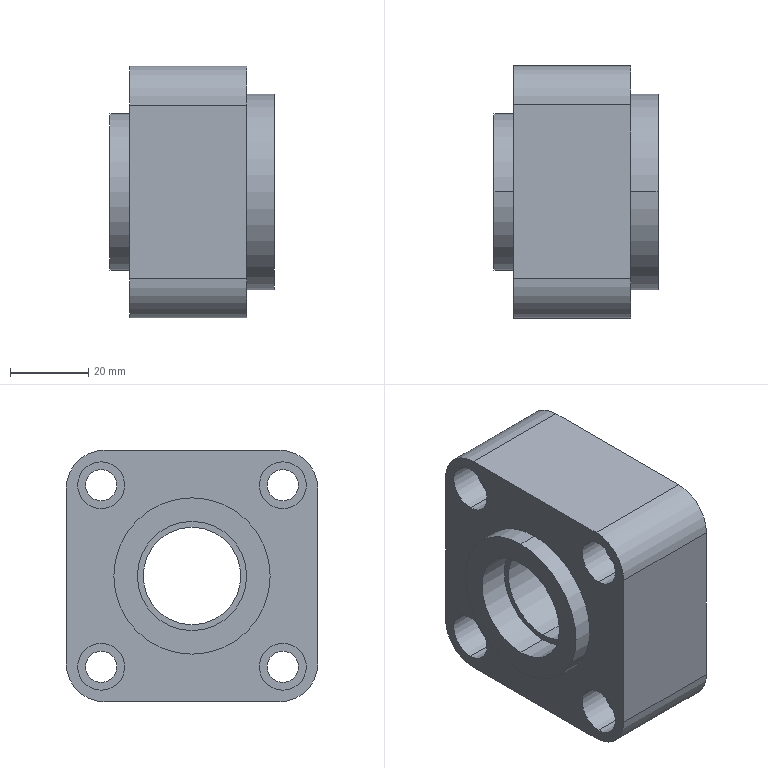Part | STEP file | 1 solid | 44 faces | box 42 x 64.5 x 64.5 mm | volume 111603 mm3 | cylinder 30 | plane 14 | commonest cylinder face diameters 8 x8 12 x8 20 x4 28 x4 25 x2 40 x2
STEP:
#1=CARTESIAN_POINT('',(-20.091,0.,-20.));
#2=VERTEX_POINT('',#1);
#3=CARTESIAN_POINT('',(-20.091,0.,20.));
#4=VERTEX_POINT('',#3);
#5=CARTESIAN_POINT('',(-20.091,0.,0.));
#6=DIRECTION('',(1.,0.,0.));
#7=DIRECTION('',(0.,0.,-1.));
#8=AXIS2_PLACEMENT_3D('',#5,#6,#7);
#9=CIRCLE('',#8,20.);
#10=EDGE_CURVE('',#2,#4,#9,.T.);
#11=ORIENTED_EDGE('',*,*,#10,.T.);
#12=CARTESIAN_POINT('',(-15.091,0.,20.));
#13=VERTEX_POINT('',#12);
#14=CARTESIAN_POINT('',(-20.091,0.,20.));
#15=DIRECTION('',(1.,0.,0.));
#16=VECTOR('',#15,1000.);
#17=LINE('',#14,#16);
#18=EDGE_CURVE('',#4,#13,#17,.T.);
#19=ORIENTED_EDGE('',*,*,#18,.T.);
#20=CARTESIAN_POINT('',(-15.091,0.,-20.));
#21=VERTEX_POINT('',#20);
#22=CARTESIAN_POINT('',(-15.091,0.,0.));
#23=DIRECTION('',(1.,0.,0.));
#24=DIRECTION('',(0.,0.,-1.));
#25=AXIS2_PLACEMENT_3D('',#22,#23,#24);
#26=CIRCLE('',#25,20.);
#27=EDGE_CURVE('',#21,#13,#26,.T.);
#28=ORIENTED_EDGE('',*,*,#27,.F.);
#29=CARTESIAN_POINT('',(-20.091,0.,-20.));
#30=DIRECTION('',(1.,0.,0.));
#31=VECTOR('',#30,1000.);
#32=LINE('',#29,#31);
#33=EDGE_CURVE('',#2,#21,#32,.T.);
#34=ORIENTED_EDGE('',*,*,#33,.F.);
#35=EDGE_LOOP('',(#11,#19,#28,#34));
#36=FACE_OUTER_BOUND('',#35,.T.);
#37=CARTESIAN_POINT('',(-20.091,0.,0.));
#38=DIRECTION('',(1.,0.,0.));
#39=DIRECTION('',(0.,0.,-1.));
#40=AXIS2_PLACEMENT_3D('',#37,#38,#39);
#41=CYLINDRICAL_SURFACE('',#40,20.);
#42=ADVANCED_FACE('',(#36),#41,.T.);
#43=CARTESIAN_POINT('',(-15.091,23.25,29.25));
#44=VERTEX_POINT('',#43);
#45=CARTESIAN_POINT('',(-15.091,23.25,17.25));
#46=VERTEX_POINT('',#45);
#47=CARTESIAN_POINT('',(-15.091,23.25,23.25));
#48=DIRECTION('',(1.,0.,0.));
#49=DIRECTION('',(0.,0.,-1.));
#50=AXIS2_PLACEMENT_3D('',#47,#48,#49);
#51=CIRCLE('',#50,6.);
#52=EDGE_CURVE('',#44,#46,#51,.T.);
#53=ORIENTED_EDGE('',*,*,#52,.F.);
#54=CARTESIAN_POINT('',(-7.091,23.25,29.25));
#55=VERTEX_POINT('',#54);
#56=CARTESIAN_POINT('',(-15.091,23.25,29.25));
#57=DIRECTION('',(1.,0.,0.));
#58=VECTOR('',#57,1000.);
#59=LINE('',#56,#58);
#60=EDGE_CURVE('',#44,#55,#59,.T.);
#61=ORIENTED_EDGE('',*,*,#60,.T.);
#62=CARTESIAN_POINT('',(-7.091,23.25,17.25));
#63=VERTEX_POINT('',#62);
#64=CARTESIAN_POINT('',(-7.091,23.25,23.25));
#65=DIRECTION('',(-1.,0.,0.));
#66=DIRECTION('',(0.,0.,-1.));
#67=AXIS2_PLACEMENT_3D('',#64,#65,#66);
#68=CIRCLE('',#67,6.);
#69=EDGE_CURVE('',#63,#55,#68,.T.);
#70=ORIENTED_EDGE('',*,*,#69,.F.);
#71=CARTESIAN_POINT('',(-15.091,23.25,17.25));
#72=DIRECTION('',(1.,0.,0.));
#73=VECTOR('',#72,1000.);
#74=LINE('',#71,#73);
#75=EDGE_CURVE('',#46,#63,#74,.T.);
#76=ORIENTED_EDGE('',*,*,#75,.F.);
#77=EDGE_LOOP('',(#53,#61,#70,#76));
#78=FACE_OUTER_BOUND('',#77,.T.);
#79=CARTESIAN_POINT('',(-15.091,23.25,23.25));
#80=DIRECTION('',(1.,0.,0.));
#81=DIRECTION('',(0.,0.,-1.));
#82=AXIS2_PLACEMENT_3D('',#79,#80,#81);
#83=CYLINDRICAL_SURFACE('',#82,6.);
#84=ADVANCED_FACE('',(#78),#83,.F.);
#85=CARTESIAN_POINT('',(-15.091,23.25,-17.25));
#86=VERTEX_POINT('',#85);
#87=CARTESIAN_POINT('',(-15.091,23.25,-29.25));
#88=VERTEX_POINT('',#87);
#89=CARTESIAN_POINT('',(-15.091,23.25,-23.25));
#90=DIRECTION('',(1.,0.,0.));
#91=DIRECTION('',(0.,0.,-1.));
#92=AXIS2_PLACEMENT_3D('',#89,#90,#91);
#93=CIRCLE('',#92,6.);
#94=EDGE_CURVE('',#86,#88,#93,.T.);
#95=ORIENTED_EDGE('',*,*,#94,.F.);
#96=CARTESIAN_POINT('',(-7.091,23.25,-17.25));
#97=VERTEX_POINT('',#96);
#98=CARTESIAN_POINT('',(-15.091,23.25,-17.25));
#99=DIRECTION('',(1.,0.,0.));
#100=VECTOR('',#99,1000.);
#101=LINE('',#98,#100);
#102=EDGE_CURVE('',#86,#97,#101,.T.);
#103=ORIENTED_EDGE('',*,*,#102,.T.);
#104=CARTESIAN_POINT('',(-7.091,23.25,-29.25));
#105=VERTEX_POINT('',#104);
#106=CARTESIAN_POINT('',(-7.091,23.25,-23.25));
#107=DIRECTION('',(-1.,0.,0.));
#108=DIRECTION('',(0.,0.,-1.));
#109=AXIS2_PLACEMENT_3D('',#106,#107,#108);
#110=CIRCLE('',#109,6.);
#111=EDGE_CURVE('',#105,#97,#110,.T.);
#112=ORIENTED_EDGE('',*,*,#111,.F.);
#113=CARTESIAN_POINT('',(-15.091,23.25,-29.25));
#114=DIRECTION('',(1.,0.,0.));
#115=VECTOR('',#114,1000.);
#116=LINE('',#113,#115);
#117=EDGE_CURVE('',#88,#105,#116,.T.);
#118=ORIENTED_EDGE('',*,*,#117,.F.);
#119=EDGE_LOOP('',(#95,#103,#112,#118));
#120=FACE_OUTER_BOUND('',#119,.T.);
#121=CARTESIAN_POINT('',(-15.091,23.25,-23.25));
#122=DIRECTION('',(1.,0.,0.));
#123=DIRECTION('',(0.,0.,-1.));
#124=AXIS2_PLACEMENT_3D('',#121,#122,#123);
#125=CYLINDRICAL_SURFACE('',#124,6.);
#126=ADVANCED_FACE('',(#120),#125,.F.);
#127=CARTESIAN_POINT('',(-15.091,-23.25,-17.25));
#128=VERTEX_POINT('',#127);
#129=CARTESIAN_POINT('',(-15.091,-23.25,-29.25));
#130=VERTEX_POINT('',#129);
#131=CARTESIAN_POINT('',(-15.091,-23.25,-23.25));
#132=DIRECTION('',(1.,0.,0.));
#133=DIRECTION('',(0.,0.,-1.));
#134=AXIS2_PLACEMENT_3D('',#131,#132,#133);
#135=CIRCLE('',#134,6.);
#136=EDGE_CURVE('',#128,#130,#135,.T.);
#137=ORIENTED_EDGE('',*,*,#136,.F.);
#138=CARTESIAN_POINT('',(-7.091,-23.25,-17.25));
#139=VERTEX_POINT('',#138);
#140=CARTESIAN_POINT('',(-15.091,-23.25,-17.25));
#141=DIRECTION('',(1.,0.,0.));
#142=VECTOR('',#141,1000.);
#143=LINE('',#140,#142);
#144=EDGE_CURVE('',#128,#139,#143,.T.);
#145=ORIENTED_EDGE('',*,*,#144,.T.);
#146=CARTESIAN_POINT('',(-7.091,-23.25,-29.25));
#147=VERTEX_POINT('',#146);
#148=CARTESIAN_POINT('',(-7.091,-23.25,-23.25));
#149=DIRECTION('',(-1.,0.,0.));
#150=DIRECTION('',(0.,0.,-1.));
#151=AXIS2_PLACEMENT_3D('',#148,#149,#150);
#152=CIRCLE('',#151,6.);
#153=EDGE_CURVE('',#147,#139,#152,.T.);
#154=ORIENTED_EDGE('',*,*,#153,.F.);
#155=CARTESIAN_POINT('',(-15.091,-23.25,-29.25));
#156=DIRECTION('',(1.,0.,0.));
#157=VECTOR('',#156,1000.);
#158=LINE('',#155,#157);
#159=EDGE_CURVE('',#130,#147,#158,.T.);
#160=ORIENTED_EDGE('',*,*,#159,.F.);
#161=EDGE_LOOP('',(#137,#145,#154,#160));
#162=FACE_OUTER_BOUND('',#161,.T.);
#163=CARTESIAN_POINT('',(-15.091,-23.25,-23.25));
#164=DIRECTION('',(1.,0.,0.));
#165=DIRECTION('',(0.,0.,-1.));
#166=AXIS2_PLACEMENT_3D('',#163,#164,#165);
#167=CYLINDRICAL_SURFACE('',#166,6.);
#168=ADVANCED_FACE('',(#162),#167,.F.);
#169=CARTESIAN_POINT('',(-15.091,-23.25,29.25));
#170=VERTEX_POINT('',#169);
#171=CARTESIAN_POINT('',(-15.091,-23.25,17.25));
#172=VERTEX_POINT('',#171);
#173=CARTESIAN_POINT('',(-15.091,-23.25,23.25));
#174=DIRECTION('',(1.,0.,0.));
#175=DIRECTION('',(0.,0.,-1.));
#176=AXIS2_PLACEMENT_3D('',#173,#174,#175);
#177=CIRCLE('',#176,6.);
#178=EDGE_CURVE('',#170,#172,#177,.T.);
#179=ORIENTED_EDGE('',*,*,#178,.F.);
#180=CARTESIAN_POINT('',(-7.091,-23.25,29.25));
#181=VERTEX_POINT('',#180);
#182=CARTESIAN_POINT('',(-15.091,-23.25,29.25));
#183=DIRECTION('',(1.,0.,0.));
#184=VECTOR('',#183,1000.);
#185=LINE('',#182,#184);
#186=EDGE_CURVE('',#170,#181,#185,.T.);
#187=ORIENTED_EDGE('',*,*,#186,.T.);
#188=CARTESIAN_POINT('',(-7.091,-23.25,17.25));
#189=VERTEX_POINT('',#188);
#190=CARTESIAN_POINT('',(-7.091,-23.25,23.25));
#191=DIRECTION('',(-1.,0.,0.));
#192=DIRECTION('',(0.,0.,-1.));
#193=AXIS2_PLACEMENT_3D('',#190,#191,#192);
#194=CIRCLE('',#193,6.);
#195=EDGE_CURVE('',#189,#181,#194,.T.);
#196=ORIENTED_EDGE('',*,*,#195,.F.);
#197=CARTESIAN_POINT('',(-15.091,-23.25,17.25));
#198=DIRECTION('',(1.,0.,0.));
#199=VECTOR('',#198,1000.);
#200=LINE('',#197,#199);
#201=EDGE_CURVE('',#172,#189,#200,.T.);
#202=ORIENTED_EDGE('',*,*,#201,.F.);
#203=EDGE_LOOP('',(#179,#187,#196,#202));
#204=FACE_OUTER_BOUND('',#203,.T.);
#205=CARTESIAN_POINT('',(-15.091,-23.25,23.25));
#206=DIRECTION('',(1.,0.,0.));
#207=DIRECTION('',(0.,0.,-1.));
#208=AXIS2_PLACEMENT_3D('',#205,#206,#207);
#209=CYLINDRICAL_SURFACE('',#208,6.);
#210=ADVANCED_FACE('',(#204),#209,.F.);
#211=CARTESIAN_POINT('',(14.909,0.,25.));
#212=VERTEX_POINT('',#211);
#213=CARTESIAN_POINT('',(14.909,0.,-25.));
#214=VERTEX_POINT('',#213);
#215=CARTESIAN_POINT('',(14.909,0.,0.));
#216=DIRECTION('',(-1.,0.,0.));
#217=DIRECTION('',(0.,0.,-1.));
#218=AXIS2_PLACEMENT_3D('',#215,#216,#217);
#219=CIRCLE('',#218,25.);
#220=EDGE_CURVE('',#212,#214,#219,.T.);
#221=ORIENTED_EDGE('',*,*,#220,.F.);
#222=CARTESIAN_POINT('',(21.909,0.,25.));
#223=VERTEX_POINT('',#222);
#224=CARTESIAN_POINT('',(14.909,0.,25.));
#225=DIRECTION('',(1.,0.,0.));
#226=VECTOR('',#225,1000.);
#227=LINE('',#224,#226);
#228=EDGE_CURVE('',#212,#223,#227,.T.);
#229=ORIENTED_EDGE('',*,*,#228,.T.);
#230=CARTESIAN_POINT('',(21.909,0.,-25.));
#231=VERTEX_POINT('',#230);
#232=CARTESIAN_POINT('',(21.909,0.,0.));
#233=DIRECTION('',(-1.,0.,0.));
#234=DIRECTION('',(0.,0.,-1.));
#235=AXIS2_PLACEMENT_3D('',#232,#233,#234);
#236=CIRCLE('',#235,25.);
#237=EDGE_CURVE('',#223,#231,#236,.T.);
#238=ORIENTED_EDGE('',*,*,#237,.T.);
#239=CARTESIAN_POINT('',(14.909,0.,-25.));
#240=DIRECTION('',(1.,0.,0.));
#241=VECTOR('',#240,1000.);
#242=LINE('',#239,#241);
#243=EDGE_CURVE('',#214,#231,#242,.T.);
#244=ORIENTED_EDGE('',*,*,#243,.F.);
#245=EDGE_LOOP('',(#221,#229,#238,#244));
#246=FACE_OUTER_BOUND('',#245,.T.);
#247=CARTESIAN_POINT('',(14.909,0.,0.));
#248=DIRECTION('',(1.,0.,0.));
#249=DIRECTION('',(0.,0.,-1.));
#250=AXIS2_PLACEMENT_3D('',#247,#248,#249);
#251=CYLINDRICAL_SURFACE('',#250,25.);
#252=ADVANCED_FACE('',(#246),#251,.T.);
#253=CARTESIAN_POINT('',(-7.091,23.25,19.25));
#254=VERTEX_POINT('',#253);
#255=CARTESIAN_POINT('',(-7.091,23.25,27.25));
#256=VERTEX_POINT('',#255);
#257=CARTESIAN_POINT('',(-7.091,23.25,23.25));
#258=DIRECTION('',(-1.,0.,0.));
#259=DIRECTION('',(0.,0.,-1.));
#260=AXIS2_PLACEMENT_3D('',#257,#258,#259);
#261=CIRCLE('',#260,4.);
#262=EDGE_CURVE('',#254,#256,#261,.T.);
#263=ORIENTED_EDGE('',*,*,#262,.T.);
#264=CARTESIAN_POINT('',(14.909,23.25,27.25));
#265=VERTEX_POINT('',#264);
#266=CARTESIAN_POINT('',(-7.091,23.25,27.25));
#267=DIRECTION('',(1.,0.,0.));
#268=VECTOR('',#267,1000.);
#269=LINE('',#266,#268);
#270=EDGE_CURVE('',#256,#265,#269,.T.);
#271=ORIENTED_EDGE('',*,*,#270,.T.);
#272=CARTESIAN_POINT('',(14.909,23.25,19.25));
#273=VERTEX_POINT('',#272);
#274=CARTESIAN_POINT('',(14.909,23.25,23.25));
#275=DIRECTION('',(-1.,0.,0.));
#276=DIRECTION('',(0.,0.,-1.));
#277=AXIS2_PLACEMENT_3D('',#274,#275,#276);
#278=CIRCLE('',#277,4.);
#279=EDGE_CURVE('',#273,#265,#278,.T.);
#280=ORIENTED_EDGE('',*,*,#279,.F.);
#281=CARTESIAN_POINT('',(-7.091,23.25,19.25));
#282=DIRECTION('',(1.,0.,0.));
#283=VECTOR('',#282,1000.);
#284=LINE('',#281,#283);
#285=EDGE_CURVE('',#254,#273,#284,.T.);
#286=ORIENTED_EDGE('',*,*,#285,.F.);
#287=EDGE_LOOP('',(#263,#271,#280,#286));
#288=FACE_OUTER_BOUND('',#287,.T.);
#289=CARTESIAN_POINT('',(-7.091,23.25,23.25));
#290=DIRECTION('',(1.,0.,0.));
#291=DIRECTION('',(0.,0.,-1.));
#292=AXIS2_PLACEMENT_3D('',#289,#290,#291);
#293=CYLINDRICAL_SURFACE('',#292,4.);
#294=ADVANCED_FACE('',(#288),#293,.F.);
#295=CARTESIAN_POINT('',(-7.091,23.25,-27.25));
#296=VERTEX_POINT('',#295);
#297=CARTESIAN_POINT('',(-7.091,23.25,-19.25));
#298=VERTEX_POINT('',#297);
#299=CARTESIAN_POINT('',(-7.091,23.25,-23.25));
#300=DIRECTION('',(-1.,0.,0.));
#301=DIRECTION('',(0.,0.,-1.));
#302=AXIS2_PLACEMENT_3D('',#299,#300,#301);
#303=CIRCLE('',#302,4.);
#304=EDGE_CURVE('',#296,#298,#303,.T.);
#305=ORIENTED_EDGE('',*,*,#304,.T.);
#306=CARTESIAN_POINT('',(14.909,23.25,-19.25));
#307=VERTEX_POINT('',#306);
#308=CARTESIAN_POINT('',(-7.091,23.25,-19.25));
#309=DIRECTION('',(1.,0.,0.));
#310=VECTOR('',#309,1000.);
#311=LINE('',#308,#310);
#312=EDGE_CURVE('',#298,#307,#311,.T.);
#313=ORIENTED_EDGE('',*,*,#312,.T.);
#314=CARTESIAN_POINT('',(14.909,23.25,-27.25));
#315=VERTEX_POINT('',#314);
#316=CARTESIAN_POINT('',(14.909,23.25,-23.25));
#317=DIRECTION('',(-1.,0.,0.));
#318=DIRECTION('',(0.,0.,-1.));
#319=AXIS2_PLACEMENT_3D('',#316,#317,#318);
#320=CIRCLE('',#319,4.);
#321=EDGE_CURVE('',#315,#307,#320,.T.);
#322=ORIENTED_EDGE('',*,*,#321,.F.);
#323=CARTESIAN_POINT('',(-7.091,23.25,-27.25));
#324=DIRECTION('',(1.,0.,0.));
#325=VECTOR('',#324,1000.);
#326=LINE('',#323,#325);
#327=EDGE_CURVE('',#296,#315,#326,.T.);
#328=ORIENTED_EDGE('',*,*,#327,.F.);
#329=EDGE_LOOP('',(#305,#313,#322,#328));
#330=FACE_OUTER_BOUND('',#329,.T.);
#331=CARTESIAN_POINT('',(-7.091,23.25,-23.25));
#332=DIRECTION('',(1.,0.,0.));
#333=DIRECTION('',(0.,0.,-1.));
#334=AXIS2_PLACEMENT_3D('',#331,#332,#333);
#335=CYLINDRICAL_SURFACE('',#334,4.);
#336=ADVANCED_FACE('',(#330),#335,.F.);
#337=CARTESIAN_POINT('',(-7.091,-23.25,-27.25));
#338=VERTEX_POINT('',#337);
#339=CARTESIAN_POINT('',(-7.091,-23.25,-19.25));
#340=VERTEX_POINT('',#339);
#341=CARTESIAN_POINT('',(-7.091,-23.25,-23.25));
#342=DIRECTION('',(-1.,0.,0.));
#343=DIRECTION('',(0.,0.,-1.));
#344=AXIS2_PLACEMENT_3D('',#341,#342,#343);
#345=CIRCLE('',#344,4.);
#346=EDGE_CURVE('',#338,#340,#345,.T.);
#347=ORIENTED_EDGE('',*,*,#346,.T.);
#348=CARTESIAN_POINT('',(14.909,-23.25,-19.25));
#349=VERTEX_POINT('',#348);
#350=CARTESIAN_POINT('',(-7.091,-23.25,-19.25));
#351=DIRECTION('',(1.,0.,0.));
#352=VECTOR('',#351,1000.);
#353=LINE('',#350,#352);
#354=EDGE_CURVE('',#340,#349,#353,.T.);
#355=ORIENTED_EDGE('',*,*,#354,.T.);
#356=CARTESIAN_POINT('',(14.909,-23.25,-27.25));
#357=VERTEX_POINT('',#356);
#358=CARTESIAN_POINT('',(14.909,-23.25,-23.25));
#359=DIRECTION('',(-1.,0.,0.));
#360=DIRECTION('',(0.,0.,-1.));
#361=AXIS2_PLACEMENT_3D('',#358,#359,#360);
#362=CIRCLE('',#361,4.);
#363=EDGE_CURVE('',#357,#349,#362,.T.);
#364=ORIENTED_EDGE('',*,*,#363,.F.);
#365=CARTESIAN_POINT('',(-7.091,-23.25,-27.25));
#366=DIRECTION('',(1.,0.,0.));
#367=VECTOR('',#366,1000.);
#368=LINE('',#365,#367);
#369=EDGE_CURVE('',#338,#357,#368,.T.);
#370=ORIENTED_EDGE('',*,*,#369,.F.);
#371=EDGE_LOOP('',(#347,#355,#364,#370));
#372=FACE_OUTER_BOUND('',#371,.T.);
#373=CARTESIAN_POINT('',(-7.091,-23.25,-23.25));
#374=DIRECTION('',(1.,0.,0.));
#375=DIRECTION('',(0.,0.,-1.));
#376=AXIS2_PLACEMENT_3D('',#373,#374,#375);
#377=CYLINDRICAL_SURFACE('',#376,4.);
#378=ADVANCED_FACE('',(#372),#377,.F.);
#379=CARTESIAN_POINT('',(-7.091,-23.25,19.25));
#380=VERTEX_POINT('',#379);
#381=CARTESIAN_POINT('',(-7.091,-23.25,27.25));
#382=VERTEX_POINT('',#381);
#383=CARTESIAN_POINT('',(-7.091,-23.25,23.25));
#384=DIRECTION('',(-1.,0.,0.));
#385=DIRECTION('',(0.,0.,-1.));
#386=AXIS2_PLACEMENT_3D('',#383,#384,#385);
#387=CIRCLE('',#386,4.);
#388=EDGE_CURVE('',#380,#382,#387,.T.);
#389=ORIENTED_EDGE('',*,*,#388,.T.);
#390=CARTESIAN_POINT('',(14.909,-23.25,27.25));
#391=VERTEX_POINT('',#390);
#392=CARTESIAN_POINT('',(-7.091,-23.25,27.25));
#393=DIRECTION('',(1.,0.,0.));
#394=VECTOR('',#393,1000.);
#395=LINE('',#392,#394);
#396=EDGE_CURVE('',#382,#391,#395,.T.);
#397=ORIENTED_EDGE('',*,*,#396,.T.);
#398=CARTESIAN_POINT('',(14.909,-23.25,19.25));
#399=VERTEX_POINT('',#398);
#400=CARTESIAN_POINT('',(14.909,-23.25,23.25));
#401=DIRECTION('',(-1.,0.,0.));
#402=DIRECTION('',(0.,0.,-1.));
#403=AXIS2_PLACEMENT_3D('',#400,#401,#402);
#404=CIRCLE('',#403,4.);
#405=EDGE_CURVE('',#399,#391,#404,.T.);
#406=ORIENTED_EDGE('',*,*,#405,.F.);
#407=CARTESIAN_POINT('',(-7.091,-23.25,19.25));
#408=DIRECTION('',(1.,0.,0.));
#409=VECTOR('',#408,1000.);
#410=LINE('',#407,#409);
#411=EDGE_CURVE('',#380,#399,#410,.T.);
#412=ORIENTED_EDGE('',*,*,#411,.F.);
#413=EDGE_LOOP('',(#389,#397,#406,#412));
#414=FACE_OUTER_BOUND('',#413,.T.);
#415=CARTESIAN_POINT('',(-7.091,-23.25,23.25));
#416=DIRECTION('',(1.,0.,0.));
#417=DIRECTION('',(0.,0.,-1.));
#418=AXIS2_PLACEMENT_3D('',#415,#416,#417);
#419=CYLINDRICAL_SURFACE('',#418,4.);
#420=ADVANCED_FACE('',(#414),#419,.F.);
#421=CARTESIAN_POINT('',(-20.091,0.,14.));
#422=VERTEX_POINT('',#421);
#423=CARTESIAN_POINT('',(-20.091,0.,-14.));
#424=VERTEX_POINT('',#423);
#425=CARTESIAN_POINT('',(-20.091,0.,0.));
#426=DIRECTION('',(1.,0.,0.));
#427=DIRECTION('',(0.,0.,-1.));
#428=AXIS2_PLACEMENT_3D('',#425,#426,#427);
#429=CIRCLE('',#428,14.);
#430=EDGE_CURVE('',#422,#424,#429,.T.);
#431=ORIENTED_EDGE('',*,*,#430,.F.);
#432=CARTESIAN_POINT('',(-12.091,0.,14.));
#433=VERTEX_POINT('',#432);
#434=CARTESIAN_POINT('',(-20.091,0.,14.));
#435=DIRECTION('',(1.,0.,0.));
#436=VECTOR('',#435,1000.);
#437=LINE('',#434,#436);
#438=EDGE_CURVE('',#422,#433,#437,.T.);
#439=ORIENTED_EDGE('',*,*,#438,.T.);
#440=CARTESIAN_POINT('',(-12.091,0.,-14.));
#441=VERTEX_POINT('',#440);
#442=CARTESIAN_POINT('',(-12.091,0.,0.));
#443=DIRECTION('',(-1.,0.,0.));
#444=DIRECTION('',(0.,0.,-1.));
#445=AXIS2_PLACEMENT_3D('',#442,#443,#444);
#446=CIRCLE('',#445,14.);
#447=EDGE_CURVE('',#441,#433,#446,.T.);
#448=ORIENTED_EDGE('',*,*,#447,.F.);
#449=CARTESIAN_POINT('',(-20.091,0.,-14.));
#450=DIRECTION('',(1.,0.,0.));
#451=VECTOR('',#450,1000.);
#452=LINE('',#449,#451);
#453=EDGE_CURVE('',#424,#441,#452,.T.);
#454=ORIENTED_EDGE('',*,*,#453,.F.);
#455=EDGE_LOOP('',(#431,#439,#448,#454));
#456=FACE_OUTER_BOUND('',#455,.T.);
#457=CARTESIAN_POINT('',(-20.091,0.,0.));
#458=DIRECTION('',(1.,0.,0.));
#459=DIRECTION('',(0.,0.,-1.));
#460=AXIS2_PLACEMENT_3D('',#457,#458,#459);
#461=CYLINDRICAL_SURFACE('',#460,14.);
#462=ADVANCED_FACE('',(#456),#461,.F.);
#463=CARTESIAN_POINT('',(13.909,0.,14.));
#464=VERTEX_POINT('',#463);
#465=CARTESIAN_POINT('',(13.909,0.,-14.));
#466=VERTEX_POINT('',#465);
#467=CARTESIAN_POINT('',(13.909,0.,0.));
#468=DIRECTION('',(1.,0.,0.));
#469=DIRECTION('',(0.,0.,-1.));
#470=AXIS2_PLACEMENT_3D('',#467,#468,#469);
#471=CIRCLE('',#470,14.);
#472=EDGE_CURVE('',#464,#466,#471,.T.);
#473=ORIENTED_EDGE('',*,*,#472,.F.);
#474=CARTESIAN_POINT('',(21.909,0.,14.));
#475=VERTEX_POINT('',#474);
#476=CARTESIAN_POINT('',(13.909,0.,14.));
#477=DIRECTION('',(1.,0.,0.));
#478=VECTOR('',#477,1000.);
#479=LINE('',#476,#478);
#480=EDGE_CURVE('',#464,#475,#479,.T.);
#481=ORIENTED_EDGE('',*,*,#480,.T.);
#482=CARTESIAN_POINT('',(21.909,0.,-14.));
#483=VERTEX_POINT('',#482);
#484=CARTESIAN_POINT('',(21.909,0.,0.));
#485=DIRECTION('',(-1.,0.,0.));
#486=DIRECTION('',(0.,0.,-1.));
#487=AXIS2_PLACEMENT_3D('',#484,#485,#486);
#488=CIRCLE('',#487,14.);
#489=EDGE_CURVE('',#483,#475,#488,.T.);
#490=ORIENTED_EDGE('',*,*,#489,.F.);
#491=CARTESIAN_POINT('',(13.909,0.,-14.));
#492=DIRECTION('',(1.,0.,0.));
#493=VECTOR('',#492,1000.);
#494=LINE('',#491,#493);
#495=EDGE_CURVE('',#466,#483,#494,.T.);
#496=ORIENTED_EDGE('',*,*,#495,.F.);
#497=EDGE_LOOP('',(#473,#481,#490,#496));
#498=FACE_OUTER_BOUND('',#497,.T.);
#499=CARTESIAN_POINT('',(13.909,0.,0.));
#500=DIRECTION('',(1.,0.,0.));
#501=DIRECTION('',(0.,0.,-1.));
#502=AXIS2_PLACEMENT_3D('',#499,#500,#501);
#503=CYLINDRICAL_SURFACE('',#502,14.);
#504=ADVANCED_FACE('',(#498),#503,.F.);
#505=CARTESIAN_POINT('',(-12.091,0.,-12.5));
#506=VERTEX_POINT('',#505);
#507=CARTESIAN_POINT('',(-12.091,0.,12.5));
#508=VERTEX_POINT('',#507);
#509=CARTESIAN_POINT('',(-12.091,0.,0.));
#510=DIRECTION('',(-1.,0.,0.));
#511=DIRECTION('',(0.,0.,-1.));
#512=AXIS2_PLACEMENT_3D('',#509,#510,#511);
#513=CIRCLE('',#512,12.5);
#514=EDGE_CURVE('',#506,#508,#513,.T.);
#515=ORIENTED_EDGE('',*,*,#514,.T.);
#516=CARTESIAN_POINT('',(13.909,0.,12.5));
#517=VERTEX_POINT('',#516);
#518=CARTESIAN_POINT('',(-12.091,0.,12.5));
#519=DIRECTION('',(1.,0.,0.));
#520=VECTOR('',#519,1000.);
#521=LINE('',#518,#520);
#522=EDGE_CURVE('',#508,#517,#521,.T.);
#523=ORIENTED_EDGE('',*,*,#522,.T.);
#524=CARTESIAN_POINT('',(13.909,0.,-12.5));
#525=VERTEX_POINT('',#524);
#526=CARTESIAN_POINT('',(13.909,0.,0.));
#527=DIRECTION('',(-1.,0.,0.));
#528=DIRECTION('',(0.,0.,-1.));
#529=AXIS2_PLACEMENT_3D('',#526,#527,#528);
#530=CIRCLE('',#529,12.5);
#531=EDGE_CURVE('',#525,#517,#530,.T.);
#532=ORIENTED_EDGE('',*,*,#531,.F.);
#533=CARTESIAN_POINT('',(-12.091,0.,-12.5));
#534=DIRECTION('',(1.,0.,0.));
#535=VECTOR('',#534,1000.);
#536=LINE('',#533,#535);
#537=EDGE_CURVE('',#506,#525,#536,.T.);
#538=ORIENTED_EDGE('',*,*,#537,.F.);
#539=EDGE_LOOP('',(#515,#523,#532,#538));
#540=FACE_OUTER_BOUND('',#539,.T.);
#541=CARTESIAN_POINT('',(-12.091,0.,0.));
#542=DIRECTION('',(1.,0.,0.));
#543=DIRECTION('',(0.,0.,-1.));
#544=AXIS2_PLACEMENT_3D('',#541,#542,#543);
#545=CYLINDRICAL_SURFACE('',#544,12.5);
#546=ADVANCED_FACE('',(#540),#545,.F.);
#547=CARTESIAN_POINT('',(-15.091,-22.25,-32.25));
#548=VERTEX_POINT('',#547);
#549=CARTESIAN_POINT('',(-15.091,-32.25,-22.25));
#550=VERTEX_POINT('',#549);
#551=CARTESIAN_POINT('',(-15.091,-22.25,-22.25));
#552=DIRECTION('',(-1.,0.,0.));
#553=DIRECTION('',(0.,0.,-1.));
#554=AXIS2_PLACEMENT_3D('',#551,#552,#553);
#555=CIRCLE('',#554,10.);
#556=EDGE_CURVE('',#548,#550,#555,.T.);
#557=ORIENTED_EDGE('',*,*,#556,.T.);
#558=CARTESIAN_POINT('',(-15.091,-32.25,22.25));
#559=VERTEX_POINT('',#558);
#560=CARTESIAN_POINT('',(-15.091,-32.25,-32.25));
#561=DIRECTION('',(0.,0.,1.));
#562=VECTOR('',#561,1000.);
#563=LINE('',#560,#562);
#564=EDGE_CURVE('',#550,#559,#563,.T.);
#565=ORIENTED_EDGE('',*,*,#564,.T.);
#566=CARTESIAN_POINT('',(-15.091,-22.25,32.25));
#567=VERTEX_POINT('',#566);
#568=CARTESIAN_POINT('',(-15.091,-22.25,22.25));
#569=DIRECTION('',(-1.,0.,0.));
#570=DIRECTION('',(0.,0.,-1.));
#571=AXIS2_PLACEMENT_3D('',#568,#569,#570);
#572=CIRCLE('',#571,10.);
#573=EDGE_CURVE('',#559,#567,#572,.T.);
#574=ORIENTED_EDGE('',*,*,#573,.T.);
#575=CARTESIAN_POINT('',(-15.091,22.25,32.25));
#576=VERTEX_POINT('',#575);
#577=CARTESIAN_POINT('',(-15.091,-32.25,32.25));
#578=DIRECTION('',(0.,1.,0.));
#579=VECTOR('',#578,1000.);
#580=LINE('',#577,#579);
#581=EDGE_CURVE('',#567,#576,#580,.T.);
#582=ORIENTED_EDGE('',*,*,#581,.T.);
#583=CARTESIAN_POINT('',(-15.091,32.25,22.25));
#584=VERTEX_POINT('',#583);
#585=CARTESIAN_POINT('',(-15.091,22.25,22.25));
#586=DIRECTION('',(-1.,0.,0.));
#587=DIRECTION('',(0.,0.,-1.));
#588=AXIS2_PLACEMENT_3D('',#585,#586,#587);
#589=CIRCLE('',#588,10.);
#590=EDGE_CURVE('',#576,#584,#589,.T.);
#591=ORIENTED_EDGE('',*,*,#590,.T.);
#592=CARTESIAN_POINT('',(-15.091,32.25,-22.25));
#593=VERTEX_POINT('',#592);
#594=CARTESIAN_POINT('',(-15.091,32.25,-32.25));
#595=DIRECTION('',(0.,0.,-1.));
#596=VECTOR('',#595,1000.);
#597=LINE('',#594,#596);
#598=EDGE_CURVE('',#584,#593,#597,.T.);
#599=ORIENTED_EDGE('',*,*,#598,.T.);
#600=CARTESIAN_POINT('',(-15.091,22.25,-32.25));
#601=VERTEX_POINT('',#600);
#602=CARTESIAN_POINT('',(-15.091,22.25,-22.25));
#603=DIRECTION('',(-1.,0.,0.));
#604=DIRECTION('',(0.,0.,-1.));
#605=AXIS2_PLACEMENT_3D('',#602,#603,#604);
#606=CIRCLE('',#605,10.);
#607=EDGE_CURVE('',#593,#601,#606,.T.);
#608=ORIENTED_EDGE('',*,*,#607,.T.);
#609=CARTESIAN_POINT('',(-15.091,-32.25,-32.25));
#610=DIRECTION('',(0.,-1.,0.));
#611=VECTOR('',#610,1000.);
#612=LINE('',#609,#611);
#613=EDGE_CURVE('',#601,#548,#612,.T.);
#614=ORIENTED_EDGE('',*,*,#613,.T.);
#615=EDGE_LOOP('',(#557,#565,#574,#582,#591,#599,#608,#614));
#616=FACE_OUTER_BOUND('',#615,.T.);
#617=ORIENTED_EDGE('',*,*,#27,.T.);
#618=CARTESIAN_POINT('',(-15.091,0.,0.));
#619=DIRECTION('',(1.,0.,0.));
#620=DIRECTION('',(0.,0.,-1.));
#621=AXIS2_PLACEMENT_3D('',#618,#619,#620);
#622=CIRCLE('',#621,20.);
#623=EDGE_CURVE('',#13,#21,#622,.T.);
#624=ORIENTED_EDGE('',*,*,#623,.T.);
#625=EDGE_LOOP('',(#617,#624));
#626=FACE_BOUND('',#625,.T.);
#627=CARTESIAN_POINT('',(-15.091,23.25,23.25));
#628=DIRECTION('',(1.,0.,0.));
#629=DIRECTION('',(0.,0.,-1.));
#630=AXIS2_PLACEMENT_3D('',#627,#628,#629);
#631=CIRCLE('',#630,6.);
#632=EDGE_CURVE('',#46,#44,#631,.T.);
#633=ORIENTED_EDGE('',*,*,#632,.T.);
#634=ORIENTED_EDGE('',*,*,#52,.T.);
#635=EDGE_LOOP('',(#633,#634));
#636=FACE_BOUND('',#635,.T.);
#637=CARTESIAN_POINT('',(-15.091,23.25,-23.25));
#638=DIRECTION('',(1.,0.,0.));
#639=DIRECTION('',(0.,0.,-1.));
#640=AXIS2_PLACEMENT_3D('',#637,#638,#639);
#641=CIRCLE('',#640,6.);
#642=EDGE_CURVE('',#88,#86,#641,.T.);
#643=ORIENTED_EDGE('',*,*,#642,.T.);
#644=ORIENTED_EDGE('',*,*,#94,.T.);
#645=EDGE_LOOP('',(#643,#644));
#646=FACE_BOUND('',#645,.T.);
#647=CARTESIAN_POINT('',(-15.091,-23.25,-23.25));
#648=DIRECTION('',(1.,0.,0.));
#649=DIRECTION('',(0.,0.,-1.));
#650=AXIS2_PLACEMENT_3D('',#647,#648,#649);
#651=CIRCLE('',#650,6.);
#652=EDGE_CURVE('',#130,#128,#651,.T.);
#653=ORIENTED_EDGE('',*,*,#652,.T.);
#654=ORIENTED_EDGE('',*,*,#136,.T.);
#655=EDGE_LOOP('',(#653,#654));
#656=FACE_BOUND('',#655,.T.);
#657=CARTESIAN_POINT('',(-15.091,-23.25,23.25));
#658=DIRECTION('',(1.,0.,0.));
#659=DIRECTION('',(0.,0.,-1.));
#660=AXIS2_PLACEMENT_3D('',#657,#658,#659);
#661=CIRCLE('',#660,6.);
#662=EDGE_CURVE('',#172,#170,#661,.T.);
#663=ORIENTED_EDGE('',*,*,#662,.T.);
#664=ORIENTED_EDGE('',*,*,#178,.T.);
#665=EDGE_LOOP('',(#663,#664));
#666=FACE_BOUND('',#665,.T.);
#667=CARTESIAN_POINT('',(-15.091,-32.25,-32.25));
#668=DIRECTION('',(-1.,0.,0.));
#669=DIRECTION('',(0.,0.,1.));
#670=AXIS2_PLACEMENT_3D('',#667,#668,#669);
#671=PLANE('',#670);
#672=ADVANCED_FACE('',(#616,#626,#636,#646,#656,#666),#671,.T.);
#673=ORIENTED_EDGE('',*,*,#564,.F.);
#674=CARTESIAN_POINT('',(14.909,-32.25,-22.25));
#675=VERTEX_POINT('',#674);
#676=CARTESIAN_POINT('',(-15.091,-32.25,-22.25));
#677=DIRECTION('',(-1.,0.,0.));
#678=VECTOR('',#677,1000.);
#679=LINE('',#676,#678);
#680=EDGE_CURVE('',#675,#550,#679,.T.);
#681=ORIENTED_EDGE('',*,*,#680,.F.);
#682=CARTESIAN_POINT('',(14.909,-32.25,22.25));
#683=VERTEX_POINT('',#682);
#684=CARTESIAN_POINT('',(14.909,-32.25,-22.25));
#685=DIRECTION('',(0.,0.,-1.));
#686=VECTOR('',#685,1000.);
#687=LINE('',#684,#686);
#688=EDGE_CURVE('',#683,#675,#687,.T.);
#689=ORIENTED_EDGE('',*,*,#688,.F.);
#690=CARTESIAN_POINT('',(-15.091,-32.25,22.25));
#691=DIRECTION('',(1.,0.,0.));
#692=VECTOR('',#691,1000.);
#693=LINE('',#690,#692);
#694=EDGE_CURVE('',#559,#683,#693,.T.);
#695=ORIENTED_EDGE('',*,*,#694,.F.);
#696=EDGE_LOOP('',(#673,#681,#689,#695));
#697=FACE_OUTER_BOUND('',#696,.T.);
#698=CARTESIAN_POINT('',(-15.091,-32.25,-22.25));
#699=DIRECTION('',(0.,1.,0.));
#700=DIRECTION('',(1.,0.,0.));
#701=AXIS2_PLACEMENT_3D('',#698,#699,#700);
#702=PLANE('',#701);
#703=ADVANCED_FACE('',(#697),#702,.F.);
#704=ORIENTED_EDGE('',*,*,#556,.F.);
#705=CARTESIAN_POINT('',(14.909,-22.25,-32.25));
#706=VERTEX_POINT('',#705);
#707=CARTESIAN_POINT('',(-15.091,-22.25,-32.25));
#708=DIRECTION('',(1.,0.,0.));
#709=VECTOR('',#708,1000.);
#710=LINE('',#707,#709);
#711=EDGE_CURVE('',#548,#706,#710,.T.);
#712=ORIENTED_EDGE('',*,*,#711,.T.);
#713=CARTESIAN_POINT('',(14.909,-22.25,-22.25));
#714=DIRECTION('',(-1.,0.,0.));
#715=DIRECTION('',(0.,0.,-1.));
#716=AXIS2_PLACEMENT_3D('',#713,#714,#715);
#717=CIRCLE('',#716,10.);
#718=EDGE_CURVE('',#706,#675,#717,.T.);
#719=ORIENTED_EDGE('',*,*,#718,.T.);
#720=ORIENTED_EDGE('',*,*,#680,.T.);
#721=EDGE_LOOP('',(#704,#712,#719,#720));
#722=FACE_OUTER_BOUND('',#721,.T.);
#723=CARTESIAN_POINT('',(-15.091,-22.25,-22.25));
#724=DIRECTION('',(1.,0.,0.));
#725=DIRECTION('',(0.,0.,-1.));
#726=AXIS2_PLACEMENT_3D('',#723,#724,#725);
#727=CYLINDRICAL_SURFACE('',#726,10.);
#728=ADVANCED_FACE('',(#722),#727,.T.);
#729=ORIENTED_EDGE('',*,*,#613,.F.);
#730=CARTESIAN_POINT('',(14.909,22.25,-32.25));
#731=VERTEX_POINT('',#730);
#732=CARTESIAN_POINT('',(-15.091,22.25,-32.25));
#733=DIRECTION('',(-1.,0.,0.));
#734=VECTOR('',#733,1000.);
#735=LINE('',#732,#734);
#736=EDGE_CURVE('',#731,#601,#735,.T.);
#737=ORIENTED_EDGE('',*,*,#736,.F.);
#738=CARTESIAN_POINT('',(14.909,-22.25,-32.25));
#739=DIRECTION('',(0.,1.,0.));
#740=VECTOR('',#739,1000.);
#741=LINE('',#738,#740);
#742=EDGE_CURVE('',#706,#731,#741,.T.);
#743=ORIENTED_EDGE('',*,*,#742,.F.);
#744=ORIENTED_EDGE('',*,*,#711,.F.);
#745=EDGE_LOOP('',(#729,#737,#743,#744));
#746=FACE_OUTER_BOUND('',#745,.T.);
#747=CARTESIAN_POINT('',(-15.091,-22.25,-32.25));
#748=DIRECTION('',(0.,0.,1.));
#749=DIRECTION('',(1.,0.,0.));
#750=AXIS2_PLACEMENT_3D('',#747,#748,#749);
#751=PLANE('',#750);
#752=ADVANCED_FACE('',(#746),#751,.F.);
#753=ORIENTED_EDGE('',*,*,#607,.F.);
#754=CARTESIAN_POINT('',(14.909,32.25,-22.25));
#755=VERTEX_POINT('',#754);
#756=CARTESIAN_POINT('',(-15.091,32.25,-22.25));
#757=DIRECTION('',(1.,0.,0.));
#758=VECTOR('',#757,1000.);
#759=LINE('',#756,#758);
#760=EDGE_CURVE('',#593,#755,#759,.T.);
#761=ORIENTED_EDGE('',*,*,#760,.T.);
#762=CARTESIAN_POINT('',(14.909,22.25,-22.25));
#763=DIRECTION('',(-1.,0.,0.));
#764=DIRECTION('',(0.,0.,-1.));
#765=AXIS2_PLACEMENT_3D('',#762,#763,#764);
#766=CIRCLE('',#765,10.);
#767=EDGE_CURVE('',#755,#731,#766,.T.);
#768=ORIENTED_EDGE('',*,*,#767,.T.);
#769=ORIENTED_EDGE('',*,*,#736,.T.);
#770=EDGE_LOOP('',(#753,#761,#768,#769));
#771=FACE_OUTER_BOUND('',#770,.T.);
#772=CARTESIAN_POINT('',(-15.091,22.25,-22.25));
#773=DIRECTION('',(1.,0.,0.));
#774=DIRECTION('',(0.,0.,-1.));
#775=AXIS2_PLACEMENT_3D('',#772,#773,#774);
#776=CYLINDRICAL_SURFACE('',#775,10.);
#777=ADVANCED_FACE('',(#771),#776,.T.);
#778=CARTESIAN_POINT('',(14.909,32.25,22.25));
#779=VERTEX_POINT('',#778);
#780=CARTESIAN_POINT('',(14.909,32.25,22.25));
#781=DIRECTION('',(0.,0.,1.));
#782=VECTOR('',#781,1000.);
#783=LINE('',#780,#782);
#784=EDGE_CURVE('',#755,#779,#783,.T.);
#785=ORIENTED_EDGE('',*,*,#784,.F.);
#786=ORIENTED_EDGE('',*,*,#760,.F.);
#787=ORIENTED_EDGE('',*,*,#598,.F.);
#788=CARTESIAN_POINT('',(-15.091,32.25,22.25));
#789=DIRECTION('',(-1.,0.,0.));
#790=VECTOR('',#789,1000.);
#791=LINE('',#788,#790);
#792=EDGE_CURVE('',#779,#584,#791,.T.);
#793=ORIENTED_EDGE('',*,*,#792,.F.);
#794=EDGE_LOOP('',(#785,#786,#787,#793));
#795=FACE_OUTER_BOUND('',#794,.T.);
#796=CARTESIAN_POINT('',(-15.091,32.25,22.25));
#797=DIRECTION('',(0.,-1.,0.));
#798=DIRECTION('',(0.,0.,-1.));
#799=AXIS2_PLACEMENT_3D('',#796,#797,#798);
#800=PLANE('',#799);
#801=ADVANCED_FACE('',(#795),#800,.F.);
#802=ORIENTED_EDGE('',*,*,#590,.F.);
#803=CARTESIAN_POINT('',(14.909,22.25,32.25));
#804=VERTEX_POINT('',#803);
#805=CARTESIAN_POINT('',(-15.091,22.25,32.25));
#806=DIRECTION('',(1.,0.,0.));
#807=VECTOR('',#806,1000.);
#808=LINE('',#805,#807);
#809=EDGE_CURVE('',#576,#804,#808,.T.);
#810=ORIENTED_EDGE('',*,*,#809,.T.);
#811=CARTESIAN_POINT('',(14.909,22.25,22.25));
#812=DIRECTION('',(-1.,0.,0.));
#813=DIRECTION('',(0.,0.,-1.));
#814=AXIS2_PLACEMENT_3D('',#811,#812,#813);
#815=CIRCLE('',#814,10.);
#816=EDGE_CURVE('',#804,#779,#815,.T.);
#817=ORIENTED_EDGE('',*,*,#816,.T.);
#818=ORIENTED_EDGE('',*,*,#792,.T.);
#819=EDGE_LOOP('',(#802,#810,#817,#818));
#820=FACE_OUTER_BOUND('',#819,.T.);
#821=CARTESIAN_POINT('',(-15.091,22.25,22.25));
#822=DIRECTION('',(1.,0.,0.));
#823=DIRECTION('',(0.,0.,-1.));
#824=AXIS2_PLACEMENT_3D('',#821,#822,#823);
#825=CYLINDRICAL_SURFACE('',#824,10.);
#826=ADVANCED_FACE('',(#820),#825,.T.);
#827=CARTESIAN_POINT('',(14.909,-22.25,32.25));
#828=VERTEX_POINT('',#827);
#829=CARTESIAN_POINT('',(14.909,-22.25,32.25));
#830=DIRECTION('',(0.,-1.,0.));
#831=VECTOR('',#830,1000.);
#832=LINE('',#829,#831);
#833=EDGE_CURVE('',#804,#828,#832,.T.);
#834=ORIENTED_EDGE('',*,*,#833,.F.);
#835=ORIENTED_EDGE('',*,*,#809,.F.);
#836=ORIENTED_EDGE('',*,*,#581,.F.);
#837=CARTESIAN_POINT('',(14.909,-22.25,32.25));
#838=DIRECTION('',(-1.,0.,0.));
#839=VECTOR('',#838,1000.);
#840=LINE('',#837,#839);
#841=EDGE_CURVE('',#828,#567,#840,.T.);
#842=ORIENTED_EDGE('',*,*,#841,.F.);
#843=EDGE_LOOP('',(#834,#835,#836,#842));
#844=FACE_OUTER_BOUND('',#843,.T.);
#845=CARTESIAN_POINT('',(14.909,-22.25,32.25));
#846=DIRECTION('',(0.,0.,-1.));
#847=DIRECTION('',(0.,-1.,0.));
#848=AXIS2_PLACEMENT_3D('',#845,#846,#847);
#849=PLANE('',#848);
#850=ADVANCED_FACE('',(#844),#849,.F.);
#851=ORIENTED_EDGE('',*,*,#573,.F.);
#852=ORIENTED_EDGE('',*,*,#694,.T.);
#853=CARTESIAN_POINT('',(14.909,-22.25,22.25));
#854=DIRECTION('',(-1.,0.,0.));
#855=DIRECTION('',(0.,0.,-1.));
#856=AXIS2_PLACEMENT_3D('',#853,#854,#855);
#857=CIRCLE('',#856,10.);
#858=EDGE_CURVE('',#683,#828,#857,.T.);
#859=ORIENTED_EDGE('',*,*,#858,.T.);
#860=ORIENTED_EDGE('',*,*,#841,.T.);
#861=EDGE_LOOP('',(#851,#852,#859,#860));
#862=FACE_OUTER_BOUND('',#861,.T.);
#863=CARTESIAN_POINT('',(-15.091,-22.25,22.25));
#864=DIRECTION('',(1.,0.,0.));
#865=DIRECTION('',(0.,0.,-1.));
#866=AXIS2_PLACEMENT_3D('',#863,#864,#865);
#867=CYLINDRICAL_SURFACE('',#866,10.);
#868=ADVANCED_FACE('',(#862),#867,.T.);
#869=ORIENTED_EDGE('',*,*,#18,.F.);
#870=CARTESIAN_POINT('',(-20.091,0.,0.));
#871=DIRECTION('',(1.,0.,0.));
#872=DIRECTION('',(0.,0.,-1.));
#873=AXIS2_PLACEMENT_3D('',#870,#871,#872);
#874=CIRCLE('',#873,20.);
#875=EDGE_CURVE('',#4,#2,#874,.T.);
#876=ORIENTED_EDGE('',*,*,#875,.T.);
#877=ORIENTED_EDGE('',*,*,#33,.T.);
#878=ORIENTED_EDGE('',*,*,#623,.F.);
#879=EDGE_LOOP('',(#869,#876,#877,#878));
#880=FACE_OUTER_BOUND('',#879,.T.);
#881=CARTESIAN_POINT('',(-20.091,0.,0.));
#882=DIRECTION('',(1.,0.,0.));
#883=DIRECTION('',(0.,0.,-1.));
#884=AXIS2_PLACEMENT_3D('',#881,#882,#883);
#885=CYLINDRICAL_SURFACE('',#884,20.);
#886=ADVANCED_FACE('',(#880),#885,.T.);
#887=ORIENTED_EDGE('',*,*,#60,.F.);
#888=ORIENTED_EDGE('',*,*,#632,.F.);
#889=ORIENTED_EDGE('',*,*,#75,.T.);
#890=CARTESIAN_POINT('',(-7.091,23.25,23.25));
#891=DIRECTION('',(-1.,0.,0.));
#892=DIRECTION('',(0.,0.,-1.));
#893=AXIS2_PLACEMENT_3D('',#890,#891,#892);
#894=CIRCLE('',#893,6.);
#895=EDGE_CURVE('',#55,#63,#894,.T.);
#896=ORIENTED_EDGE('',*,*,#895,.F.);
#897=EDGE_LOOP('',(#887,#888,#889,#896));
#898=FACE_OUTER_BOUND('',#897,.T.);
#899=CARTESIAN_POINT('',(-15.091,23.25,23.25));
#900=DIRECTION('',(1.,0.,0.));
#901=DIRECTION('',(0.,0.,-1.));
#902=AXIS2_PLACEMENT_3D('',#899,#900,#901);
#903=CYLINDRICAL_SURFACE('',#902,6.);
#904=ADVANCED_FACE('',(#898),#903,.F.);
#905=ORIENTED_EDGE('',*,*,#102,.F.);
#906=ORIENTED_EDGE('',*,*,#642,.F.);
#907=ORIENTED_EDGE('',*,*,#117,.T.);
#908=CARTESIAN_POINT('',(-7.091,23.25,-23.25));
#909=DIRECTION('',(-1.,0.,0.));
#910=DIRECTION('',(0.,0.,-1.));
#911=AXIS2_PLACEMENT_3D('',#908,#909,#910);
#912=CIRCLE('',#911,6.);
#913=EDGE_CURVE('',#97,#105,#912,.T.);
#914=ORIENTED_EDGE('',*,*,#913,.F.);
#915=EDGE_LOOP('',(#905,#906,#907,#914));
#916=FACE_OUTER_BOUND('',#915,.T.);
#917=CARTESIAN_POINT('',(-15.091,23.25,-23.25));
#918=DIRECTION('',(1.,0.,0.));
#919=DIRECTION('',(0.,0.,-1.));
#920=AXIS2_PLACEMENT_3D('',#917,#918,#919);
#921=CYLINDRICAL_SURFACE('',#920,6.);
#922=ADVANCED_FACE('',(#916),#921,.F.);
#923=ORIENTED_EDGE('',*,*,#144,.F.);
#924=ORIENTED_EDGE('',*,*,#652,.F.);
#925=ORIENTED_EDGE('',*,*,#159,.T.);
#926=CARTESIAN_POINT('',(-7.091,-23.25,-23.25));
#927=DIRECTION('',(-1.,0.,0.));
#928=DIRECTION('',(0.,0.,-1.));
#929=AXIS2_PLACEMENT_3D('',#926,#927,#928);
#930=CIRCLE('',#929,6.);
#931=EDGE_CURVE('',#139,#147,#930,.T.);
#932=ORIENTED_EDGE('',*,*,#931,.F.);
#933=EDGE_LOOP('',(#923,#924,#925,#932));
#934=FACE_OUTER_BOUND('',#933,.T.);
#935=CARTESIAN_POINT('',(-15.091,-23.25,-23.25));
#936=DIRECTION('',(1.,0.,0.));
#937=DIRECTION('',(0.,0.,-1.));
#938=AXIS2_PLACEMENT_3D('',#935,#936,#937);
#939=CYLINDRICAL_SURFACE('',#938,6.);
#940=ADVANCED_FACE('',(#934),#939,.F.);
#941=ORIENTED_EDGE('',*,*,#186,.F.);
#942=ORIENTED_EDGE('',*,*,#662,.F.);
#943=ORIENTED_EDGE('',*,*,#201,.T.);
#944=CARTESIAN_POINT('',(-7.091,-23.25,23.25));
#945=DIRECTION('',(-1.,0.,0.));
#946=DIRECTION('',(0.,0.,-1.));
#947=AXIS2_PLACEMENT_3D('',#944,#945,#946);
#948=CIRCLE('',#947,6.);
#949=EDGE_CURVE('',#181,#189,#948,.T.);
#950=ORIENTED_EDGE('',*,*,#949,.F.);
#951=EDGE_LOOP('',(#941,#942,#943,#950));
#952=FACE_OUTER_BOUND('',#951,.T.);
#953=CARTESIAN_POINT('',(-15.091,-23.25,23.25));
#954=DIRECTION('',(1.,0.,0.));
#955=DIRECTION('',(0.,0.,-1.));
#956=AXIS2_PLACEMENT_3D('',#953,#954,#955);
#957=CYLINDRICAL_SURFACE('',#956,6.);
#958=ADVANCED_FACE('',(#952),#957,.F.);
#959=ORIENTED_EDGE('',*,*,#816,.F.);
#960=ORIENTED_EDGE('',*,*,#833,.T.);
#961=ORIENTED_EDGE('',*,*,#858,.F.);
#962=ORIENTED_EDGE('',*,*,#688,.T.);
#963=ORIENTED_EDGE('',*,*,#718,.F.);
#964=ORIENTED_EDGE('',*,*,#742,.T.);
#965=ORIENTED_EDGE('',*,*,#767,.F.);
#966=ORIENTED_EDGE('',*,*,#784,.T.);
#967=EDGE_LOOP('',(#959,#960,#961,#962,#963,#964,#965,#966));
#968=FACE_OUTER_BOUND('',#967,.T.);
#969=CARTESIAN_POINT('',(14.909,0.,0.));
#970=DIRECTION('',(-1.,0.,0.));
#971=DIRECTION('',(0.,0.,-1.));
#972=AXIS2_PLACEMENT_3D('',#969,#970,#971);
#973=CIRCLE('',#972,25.);
#974=EDGE_CURVE('',#214,#212,#973,.T.);
#975=ORIENTED_EDGE('',*,*,#974,.T.);
#976=ORIENTED_EDGE('',*,*,#220,.T.);
#977=EDGE_LOOP('',(#975,#976));
#978=FACE_BOUND('',#977,.T.);
#979=ORIENTED_EDGE('',*,*,#279,.T.);
#980=CARTESIAN_POINT('',(14.909,23.25,23.25));
#981=DIRECTION('',(-1.,0.,0.));
#982=DIRECTION('',(0.,0.,-1.));
#983=AXIS2_PLACEMENT_3D('',#980,#981,#982);
#984=CIRCLE('',#983,4.);
#985=EDGE_CURVE('',#265,#273,#984,.T.);
#986=ORIENTED_EDGE('',*,*,#985,.T.);
#987=EDGE_LOOP('',(#979,#986));
#988=FACE_BOUND('',#987,.T.);
#989=ORIENTED_EDGE('',*,*,#321,.T.);
#990=CARTESIAN_POINT('',(14.909,23.25,-23.25));
#991=DIRECTION('',(-1.,0.,0.));
#992=DIRECTION('',(0.,0.,-1.));
#993=AXIS2_PLACEMENT_3D('',#990,#991,#992);
#994=CIRCLE('',#993,4.);
#995=EDGE_CURVE('',#307,#315,#994,.T.);
#996=ORIENTED_EDGE('',*,*,#995,.T.);
#997=EDGE_LOOP('',(#989,#996));
#998=FACE_BOUND('',#997,.T.);
#999=ORIENTED_EDGE('',*,*,#363,.T.);
#1000=CARTESIAN_POINT('',(14.909,-23.25,-23.25));
#1001=DIRECTION('',(-1.,0.,0.));
#1002=DIRECTION('',(0.,0.,-1.));
#1003=AXIS2_PLACEMENT_3D('',#1000,#1001,#1002);
#1004=CIRCLE('',#1003,4.);
#1005=EDGE_CURVE('',#349,#357,#1004,.T.);
#1006=ORIENTED_EDGE('',*,*,#1005,.T.);
#1007=EDGE_LOOP('',(#999,#1006));
#1008=FACE_BOUND('',#1007,.T.);
#1009=ORIENTED_EDGE('',*,*,#405,.T.);
#1010=CARTESIAN_POINT('',(14.909,-23.25,23.25));
#1011=DIRECTION('',(-1.,0.,0.));
#1012=DIRECTION('',(0.,0.,-1.));
#1013=AXIS2_PLACEMENT_3D('',#1010,#1011,#1012);
#1014=CIRCLE('',#1013,4.);
#1015=EDGE_CURVE('',#391,#399,#1014,.T.);
#1016=ORIENTED_EDGE('',*,*,#1015,.T.);
#1017=EDGE_LOOP('',(#1009,#1016));
#1018=FACE_BOUND('',#1017,.T.);
#1019=CARTESIAN_POINT('',(14.909,-32.25,32.25));
#1020=DIRECTION('',(1.,0.,0.));
#1021=DIRECTION('',(0.,1.,0.));
#1022=AXIS2_PLACEMENT_3D('',#1019,#1020,#1021);
#1023=PLANE('',#1022);
#1024=ADVANCED_FACE('',(#968,#978,#988,#998,#1008,#1018),#1023,.T.);
#1025=ORIENTED_EDGE('',*,*,#10,.F.);
#1026=ORIENTED_EDGE('',*,*,#875,.F.);
#1027=EDGE_LOOP('',(#1025,#1026));
#1028=FACE_OUTER_BOUND('',#1027,.T.);
#1029=CARTESIAN_POINT('',(-20.091,0.,0.));
#1030=DIRECTION('',(1.,0.,0.));
#1031=DIRECTION('',(0.,0.,-1.));
#1032=AXIS2_PLACEMENT_3D('',#1029,#1030,#1031);
#1033=CIRCLE('',#1032,14.);
#1034=EDGE_CURVE('',#424,#422,#1033,.T.);
#1035=ORIENTED_EDGE('',*,*,#1034,.T.);
#1036=ORIENTED_EDGE('',*,*,#430,.T.);
#1037=EDGE_LOOP('',(#1035,#1036));
#1038=FACE_BOUND('',#1037,.T.);
#1039=CARTESIAN_POINT('',(-20.091,-20.,-20.4));
#1040=DIRECTION('',(-1.,0.,0.));
#1041=DIRECTION('',(0.,0.,1.));
#1042=AXIS2_PLACEMENT_3D('',#1039,#1040,#1041);
#1043=PLANE('',#1042);
#1044=ADVANCED_FACE('',(#1028,#1038),#1043,.T.);
#1045=ORIENTED_EDGE('',*,*,#69,.T.);
#1046=ORIENTED_EDGE('',*,*,#895,.T.);
#1047=EDGE_LOOP('',(#1045,#1046));
#1048=FACE_OUTER_BOUND('',#1047,.T.);
#1049=ORIENTED_EDGE('',*,*,#262,.F.);
#1050=CARTESIAN_POINT('',(-7.091,23.25,23.25));
#1051=DIRECTION('',(-1.,0.,0.));
#1052=DIRECTION('',(0.,0.,-1.));
#1053=AXIS2_PLACEMENT_3D('',#1050,#1051,#1052);
#1054=CIRCLE('',#1053,4.);
#1055=EDGE_CURVE('',#256,#254,#1054,.T.);
#1056=ORIENTED_EDGE('',*,*,#1055,.F.);
#1057=EDGE_LOOP('',(#1049,#1056));
#1058=FACE_BOUND('',#1057,.T.);
#1059=CARTESIAN_POINT('',(-7.091,17.13,29.25));
#1060=DIRECTION('',(1.,0.,0.));
#1061=DIRECTION('',(0.,1.,0.));
#1062=AXIS2_PLACEMENT_3D('',#1059,#1060,#1061);
#1063=PLANE('',#1062);
#1064=ADVANCED_FACE('',(#1048,#1058),#1063,.F.);
#1065=ORIENTED_EDGE('',*,*,#111,.T.);
#1066=ORIENTED_EDGE('',*,*,#913,.T.);
#1067=EDGE_LOOP('',(#1065,#1066));
#1068=FACE_OUTER_BOUND('',#1067,.T.);
#1069=ORIENTED_EDGE('',*,*,#304,.F.);
#1070=CARTESIAN_POINT('',(-7.091,23.25,-23.25));
#1071=DIRECTION('',(-1.,0.,0.));
#1072=DIRECTION('',(0.,0.,-1.));
#1073=AXIS2_PLACEMENT_3D('',#1070,#1071,#1072);
#1074=CIRCLE('',#1073,4.);
#1075=EDGE_CURVE('',#298,#296,#1074,.T.);
#1076=ORIENTED_EDGE('',*,*,#1075,.F.);
#1077=EDGE_LOOP('',(#1069,#1076));
#1078=FACE_BOUND('',#1077,.T.);
#1079=CARTESIAN_POINT('',(-7.091,17.13,-17.25));
#1080=DIRECTION('',(1.,0.,0.));
#1081=DIRECTION('',(0.,1.,0.));
#1082=AXIS2_PLACEMENT_3D('',#1079,#1080,#1081);
#1083=PLANE('',#1082);
#1084=ADVANCED_FACE('',(#1068,#1078),#1083,.F.);
#1085=ORIENTED_EDGE('',*,*,#153,.T.);
#1086=ORIENTED_EDGE('',*,*,#931,.T.);
#1087=EDGE_LOOP('',(#1085,#1086));
#1088=FACE_OUTER_BOUND('',#1087,.T.);
#1089=ORIENTED_EDGE('',*,*,#346,.F.);
#1090=CARTESIAN_POINT('',(-7.091,-23.25,-23.25));
#1091=DIRECTION('',(-1.,0.,0.));
#1092=DIRECTION('',(0.,0.,-1.));
#1093=AXIS2_PLACEMENT_3D('',#1090,#1091,#1092);
#1094=CIRCLE('',#1093,4.);
#1095=EDGE_CURVE('',#340,#338,#1094,.T.);
#1096=ORIENTED_EDGE('',*,*,#1095,.F.);
#1097=EDGE_LOOP('',(#1089,#1096));
#1098=FACE_BOUND('',#1097,.T.);
#1099=CARTESIAN_POINT('',(-7.091,-29.37,-17.25));
#1100=DIRECTION('',(1.,0.,0.));
#1101=DIRECTION('',(0.,1.,0.));
#1102=AXIS2_PLACEMENT_3D('',#1099,#1100,#1101);
#1103=PLANE('',#1102);
#1104=ADVANCED_FACE('',(#1088,#1098),#1103,.F.);
#1105=ORIENTED_EDGE('',*,*,#195,.T.);
#1106=ORIENTED_EDGE('',*,*,#949,.T.);
#1107=EDGE_LOOP('',(#1105,#1106));
#1108=FACE_OUTER_BOUND('',#1107,.T.);
#1109=ORIENTED_EDGE('',*,*,#388,.F.);
#1110=CARTESIAN_POINT('',(-7.091,-23.25,23.25));
#1111=DIRECTION('',(-1.,0.,0.));
#1112=DIRECTION('',(0.,0.,-1.));
#1113=AXIS2_PLACEMENT_3D('',#1110,#1111,#1112);
#1114=CIRCLE('',#1113,4.);
#1115=EDGE_CURVE('',#382,#380,#1114,.T.);
#1116=ORIENTED_EDGE('',*,*,#1115,.F.);
#1117=EDGE_LOOP('',(#1109,#1116));
#1118=FACE_BOUND('',#1117,.T.);
#1119=CARTESIAN_POINT('',(-7.091,-29.37,29.25));
#1120=DIRECTION('',(1.,0.,0.));
#1121=DIRECTION('',(0.,1.,0.));
#1122=AXIS2_PLACEMENT_3D('',#1119,#1120,#1121);
#1123=PLANE('',#1122);
#1124=ADVANCED_FACE('',(#1108,#1118),#1123,.F.);
#1125=ORIENTED_EDGE('',*,*,#228,.F.);
#1126=ORIENTED_EDGE('',*,*,#974,.F.);
#1127=ORIENTED_EDGE('',*,*,#243,.T.);
#1128=CARTESIAN_POINT('',(21.909,0.,0.));
#1129=DIRECTION('',(-1.,0.,0.));
#1130=DIRECTION('',(0.,0.,-1.));
#1131=AXIS2_PLACEMENT_3D('',#1128,#1129,#1130);
#1132=CIRCLE('',#1131,25.);
#1133=EDGE_CURVE('',#231,#223,#1132,.T.);
#1134=ORIENTED_EDGE('',*,*,#1133,.T.);
#1135=EDGE_LOOP('',(#1125,#1126,#1127,#1134));
#1136=FACE_OUTER_BOUND('',#1135,.T.);
#1137=CARTESIAN_POINT('',(14.909,0.,0.));
#1138=DIRECTION('',(1.,0.,0.));
#1139=DIRECTION('',(0.,0.,-1.));
#1140=AXIS2_PLACEMENT_3D('',#1137,#1138,#1139);
#1141=CYLINDRICAL_SURFACE('',#1140,25.);
#1142=ADVANCED_FACE('',(#1136),#1141,.T.);
#1143=ORIENTED_EDGE('',*,*,#270,.F.);
#1144=ORIENTED_EDGE('',*,*,#1055,.T.);
#1145=ORIENTED_EDGE('',*,*,#285,.T.);
#1146=ORIENTED_EDGE('',*,*,#985,.F.);
#1147=EDGE_LOOP('',(#1143,#1144,#1145,#1146));
#1148=FACE_OUTER_BOUND('',#1147,.T.);
#1149=CARTESIAN_POINT('',(-7.091,23.25,23.25));
#1150=DIRECTION('',(1.,0.,0.));
#1151=DIRECTION('',(0.,0.,-1.));
#1152=AXIS2_PLACEMENT_3D('',#1149,#1150,#1151);
#1153=CYLINDRICAL_SURFACE('',#1152,4.);
#1154=ADVANCED_FACE('',(#1148),#1153,.F.);
#1155=ORIENTED_EDGE('',*,*,#312,.F.);
#1156=ORIENTED_EDGE('',*,*,#1075,.T.);
#1157=ORIENTED_EDGE('',*,*,#327,.T.);
#1158=ORIENTED_EDGE('',*,*,#995,.F.);
#1159=EDGE_LOOP('',(#1155,#1156,#1157,#1158));
#1160=FACE_OUTER_BOUND('',#1159,.T.);
#1161=CARTESIAN_POINT('',(-7.091,23.25,-23.25));
#1162=DIRECTION('',(1.,0.,0.));
#1163=DIRECTION('',(0.,0.,-1.));
#1164=AXIS2_PLACEMENT_3D('',#1161,#1162,#1163);
#1165=CYLINDRICAL_SURFACE('',#1164,4.);
#1166=ADVANCED_FACE('',(#1160),#1165,.F.);
#1167=ORIENTED_EDGE('',*,*,#354,.F.);
#1168=ORIENTED_EDGE('',*,*,#1095,.T.);
#1169=ORIENTED_EDGE('',*,*,#369,.T.);
#1170=ORIENTED_EDGE('',*,*,#1005,.F.);
#1171=EDGE_LOOP('',(#1167,#1168,#1169,#1170));
#1172=FACE_OUTER_BOUND('',#1171,.T.);
#1173=CARTESIAN_POINT('',(-7.091,-23.25,-23.25));
#1174=DIRECTION('',(1.,0.,0.));
#1175=DIRECTION('',(0.,0.,-1.));
#1176=AXIS2_PLACEMENT_3D('',#1173,#1174,#1175);
#1177=CYLINDRICAL_SURFACE('',#1176,4.);
#1178=ADVANCED_FACE('',(#1172),#1177,.F.);
#1179=ORIENTED_EDGE('',*,*,#396,.F.);
#1180=ORIENTED_EDGE('',*,*,#1115,.T.);
#1181=ORIENTED_EDGE('',*,*,#411,.T.);
#1182=ORIENTED_EDGE('',*,*,#1015,.F.);
#1183=EDGE_LOOP('',(#1179,#1180,#1181,#1182));
#1184=FACE_OUTER_BOUND('',#1183,.T.);
#1185=CARTESIAN_POINT('',(-7.091,-23.25,23.25));
#1186=DIRECTION('',(1.,0.,0.));
#1187=DIRECTION('',(0.,0.,-1.));
#1188=AXIS2_PLACEMENT_3D('',#1185,#1186,#1187);
#1189=CYLINDRICAL_SURFACE('',#1188,4.);
#1190=ADVANCED_FACE('',(#1184),#1189,.F.);
#1191=ORIENTED_EDGE('',*,*,#438,.F.);
#1192=ORIENTED_EDGE('',*,*,#1034,.F.);
#1193=ORIENTED_EDGE('',*,*,#453,.T.);
#1194=CARTESIAN_POINT('',(-12.091,0.,0.));
#1195=DIRECTION('',(-1.,0.,0.));
#1196=DIRECTION('',(0.,0.,-1.));
#1197=AXIS2_PLACEMENT_3D('',#1194,#1195,#1196);
#1198=CIRCLE('',#1197,14.);
#1199=EDGE_CURVE('',#433,#441,#1198,.T.);
#1200=ORIENTED_EDGE('',*,*,#1199,.F.);
#1201=EDGE_LOOP('',(#1191,#1192,#1193,#1200));
#1202=FACE_OUTER_BOUND('',#1201,.T.);
#1203=CARTESIAN_POINT('',(-20.091,0.,0.));
#1204=DIRECTION('',(1.,0.,0.));
#1205=DIRECTION('',(0.,0.,-1.));
#1206=AXIS2_PLACEMENT_3D('',#1203,#1204,#1205);
#1207=CYLINDRICAL_SURFACE('',#1206,14.);
#1208=ADVANCED_FACE('',(#1202),#1207,.F.);
#1209=ORIENTED_EDGE('',*,*,#1133,.F.);
#1210=ORIENTED_EDGE('',*,*,#237,.F.);
#1211=EDGE_LOOP('',(#1209,#1210));
#1212=FACE_OUTER_BOUND('',#1211,.T.);
#1213=ORIENTED_EDGE('',*,*,#489,.T.);
#1214=CARTESIAN_POINT('',(21.909,0.,0.));
#1215=DIRECTION('',(-1.,0.,0.));
#1216=DIRECTION('',(0.,0.,-1.));
#1217=AXIS2_PLACEMENT_3D('',#1214,#1215,#1216);
#1218=CIRCLE('',#1217,14.);
#1219=EDGE_CURVE('',#475,#483,#1218,.T.);
#1220=ORIENTED_EDGE('',*,*,#1219,.T.);
#1221=EDGE_LOOP('',(#1213,#1220));
#1222=FACE_BOUND('',#1221,.T.);
#1223=CARTESIAN_POINT('',(21.909,-25.,25.5));
#1224=DIRECTION('',(1.,0.,0.));
#1225=DIRECTION('',(0.,1.,0.));
#1226=AXIS2_PLACEMENT_3D('',#1223,#1224,#1225);
#1227=PLANE('',#1226);
#1228=ADVANCED_FACE('',(#1212,#1222),#1227,.T.);
#1229=ORIENTED_EDGE('',*,*,#447,.T.);
#1230=ORIENTED_EDGE('',*,*,#1199,.T.);
#1231=EDGE_LOOP('',(#1229,#1230));
#1232=FACE_OUTER_BOUND('',#1231,.T.);
#1233=ORIENTED_EDGE('',*,*,#514,.F.);
#1234=CARTESIAN_POINT('',(-12.091,0.,0.));
#1235=DIRECTION('',(-1.,0.,0.));
#1236=DIRECTION('',(0.,0.,-1.));
#1237=AXIS2_PLACEMENT_3D('',#1234,#1235,#1236);
#1238=CIRCLE('',#1237,12.5);
#1239=EDGE_CURVE('',#508,#506,#1238,.T.);
#1240=ORIENTED_EDGE('',*,*,#1239,.F.);
#1241=EDGE_LOOP('',(#1233,#1240));
#1242=FACE_BOUND('',#1241,.T.);
#1243=CARTESIAN_POINT('',(-12.091,-14.28,14.));
#1244=DIRECTION('',(1.,0.,0.));
#1245=DIRECTION('',(0.,1.,0.));
#1246=AXIS2_PLACEMENT_3D('',#1243,#1244,#1245);
#1247=PLANE('',#1246);
#1248=ADVANCED_FACE('',(#1232,#1242),#1247,.F.);
#1249=ORIENTED_EDGE('',*,*,#480,.F.);
#1250=CARTESIAN_POINT('',(13.909,0.,0.));
#1251=DIRECTION('',(1.,0.,0.));
#1252=DIRECTION('',(0.,0.,-1.));
#1253=AXIS2_PLACEMENT_3D('',#1250,#1251,#1252);
#1254=CIRCLE('',#1253,14.);
#1255=EDGE_CURVE('',#466,#464,#1254,.T.);
#1256=ORIENTED_EDGE('',*,*,#1255,.F.);
#1257=ORIENTED_EDGE('',*,*,#495,.T.);
#1258=ORIENTED_EDGE('',*,*,#1219,.F.);
#1259=EDGE_LOOP('',(#1249,#1256,#1257,#1258));
#1260=FACE_OUTER_BOUND('',#1259,.T.);
#1261=CARTESIAN_POINT('',(13.909,0.,0.));
#1262=DIRECTION('',(1.,0.,0.));
#1263=DIRECTION('',(0.,0.,-1.));
#1264=AXIS2_PLACEMENT_3D('',#1261,#1262,#1263);
#1265=CYLINDRICAL_SURFACE('',#1264,14.);
#1266=ADVANCED_FACE('',(#1260),#1265,.F.);
#1267=ORIENTED_EDGE('',*,*,#522,.F.);
#1268=ORIENTED_EDGE('',*,*,#1239,.T.);
#1269=ORIENTED_EDGE('',*,*,#537,.T.);
#1270=CARTESIAN_POINT('',(13.909,0.,0.));
#1271=DIRECTION('',(-1.,0.,0.));
#1272=DIRECTION('',(0.,0.,-1.));
#1273=AXIS2_PLACEMENT_3D('',#1270,#1271,#1272);
#1274=CIRCLE('',#1273,12.5);
#1275=EDGE_CURVE('',#517,#525,#1274,.T.);
#1276=ORIENTED_EDGE('',*,*,#1275,.F.);
#1277=EDGE_LOOP('',(#1267,#1268,#1269,#1276));
#1278=FACE_OUTER_BOUND('',#1277,.T.);
#1279=CARTESIAN_POINT('',(-12.091,0.,0.));
#1280=DIRECTION('',(1.,0.,0.));
#1281=DIRECTION('',(0.,0.,-1.));
#1282=AXIS2_PLACEMENT_3D('',#1279,#1280,#1281);
#1283=CYLINDRICAL_SURFACE('',#1282,12.5);
#1284=ADVANCED_FACE('',(#1278),#1283,.F.);
#1285=ORIENTED_EDGE('',*,*,#1255,.T.);
#1286=ORIENTED_EDGE('',*,*,#472,.T.);
#1287=EDGE_LOOP('',(#1285,#1286));
#1288=FACE_OUTER_BOUND('',#1287,.T.);
#1289=ORIENTED_EDGE('',*,*,#531,.T.);
#1290=ORIENTED_EDGE('',*,*,#1275,.T.);
#1291=EDGE_LOOP('',(#1289,#1290));
#1292=FACE_BOUND('',#1291,.T.);
#1293=CARTESIAN_POINT('',(13.909,-14.,-14.28));
#1294=DIRECTION('',(1.,0.,0.));
#1295=DIRECTION('',(0.,1.,0.));
#1296=AXIS2_PLACEMENT_3D('',#1293,#1294,#1295);
#1297=PLANE('',#1296);
#1298=ADVANCED_FACE('',(#1288,#1292),#1297,.T.);
#1299=CLOSED_SHELL('',(#42,#84,#126,#168,#210,#252,#294,#336,#378,#420,#462,#504,#546,#672,#703,#728,#752,#777,#801,#826,#850,#868,#886,#904,#922,#940,#958,#1024,#1044,#1064,#1084,#1104,#1124,#1142,#1154,#1166,#1178,#1190,#1208,#1228,#1248,#1266,#1284,#1298));
#1300=MANIFOLD_SOLID_BREP('',#1299);
#1301=CARTESIAN_POINT('',(0.,0.,0.));
#1302=DIRECTION('',(0.,0.,1.));
#1303=DIRECTION('',(1.,0.,0.));
#1304=AXIS2_PLACEMENT_3D('',#1301,#1302,#1303);
#1305=(LENGTH_UNIT()NAMED_UNIT(*)SI_UNIT(.MILLI.,.METRE.));
#1306=UNCERTAINTY_MEASURE_WITH_UNIT(LENGTH_MEASURE(0.00001),#1305,'','');
#1307=(NAMED_UNIT(*)PLANE_ANGLE_UNIT()SI_UNIT($,.RADIAN.));
#1308=(NAMED_UNIT(*)SI_UNIT($,.STERADIAN.)SOLID_ANGLE_UNIT());
#1309=(GEOMETRIC_REPRESENTATION_CONTEXT(3)GLOBAL_UNCERTAINTY_ASSIGNED_CONTEXT((#1306))GLOBAL_UNIT_ASSIGNED_CONTEXT((#1305,#1307,#1308))REPRESENTATION_CONTEXT('',''));
#1310=ADVANCED_BREP_SHAPE_REPRESENTATION('',(#1300,#1304),#1309);